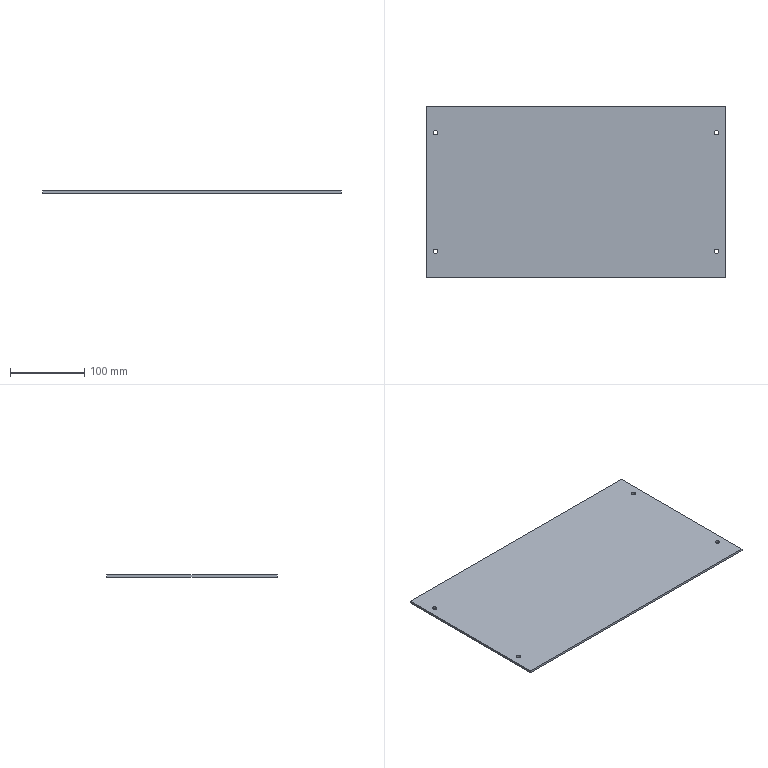Part | STEP file | Guard 7 | 1 solid | 14 faces | box 402 x 230 x 3 mm | volume 277041 mm3 | cylinder 8 | plane 6 | commonest cylinder face diameters 6 x8
STEP:
#1=CARTESIAN_POINT('',(192.,-80.,0.));
#2=VERTEX_POINT('',#1);
#3=CARTESIAN_POINT('',(186.,-80.,0.));
#4=VERTEX_POINT('',#3);
#5=CARTESIAN_POINT('',(189.,-80.,0.));
#6=DIRECTION('',(0.,0.,-1.));
#7=DIRECTION('',(1.,0.,0.));
#8=AXIS2_PLACEMENT_3D('',#5,#6,#7);
#9=CIRCLE('',#8,3.);
#10=EDGE_CURVE('',#2,#4,#9,.T.);
#11=ORIENTED_EDGE('',*,*,#10,.T.);
#12=CARTESIAN_POINT('',(186.,-80.,3.));
#13=VERTEX_POINT('',#12);
#14=CARTESIAN_POINT('',(186.,-80.,-7.));
#15=DIRECTION('',(0.,0.,1.));
#16=VECTOR('',#15,1000.);
#17=LINE('',#14,#16);
#18=EDGE_CURVE('',#4,#13,#17,.T.);
#19=ORIENTED_EDGE('',*,*,#18,.T.);
#20=CARTESIAN_POINT('',(192.,-80.,3.));
#21=VERTEX_POINT('',#20);
#22=CARTESIAN_POINT('',(189.,-80.,3.));
#23=DIRECTION('',(0.,0.,-1.));
#24=DIRECTION('',(-1.,0.,0.));
#25=AXIS2_PLACEMENT_3D('',#22,#23,#24);
#26=CIRCLE('',#25,3.);
#27=EDGE_CURVE('',#21,#13,#26,.T.);
#28=ORIENTED_EDGE('',*,*,#27,.F.);
#29=CARTESIAN_POINT('',(192.,-80.,-7.));
#30=DIRECTION('',(0.,0.,1.));
#31=VECTOR('',#30,1000.);
#32=LINE('',#29,#31);
#33=EDGE_CURVE('',#2,#21,#32,.T.);
#34=ORIENTED_EDGE('',*,*,#33,.F.);
#35=EDGE_LOOP('',(#11,#19,#28,#34));
#36=FACE_OUTER_BOUND('',#35,.T.);
#37=CARTESIAN_POINT('',(189.,-80.,-7.));
#38=DIRECTION('',(0.,0.,1.));
#39=DIRECTION('',(1.,0.,0.));
#40=AXIS2_PLACEMENT_3D('',#37,#38,#39);
#41=CYLINDRICAL_SURFACE('',#40,3.);
#42=ADVANCED_FACE('',(#36),#41,.F.);
#43=CARTESIAN_POINT('',(192.,80.,0.));
#44=VERTEX_POINT('',#43);
#45=CARTESIAN_POINT('',(186.,80.,0.));
#46=VERTEX_POINT('',#45);
#47=CARTESIAN_POINT('',(189.,80.,0.));
#48=DIRECTION('',(0.,0.,-1.));
#49=DIRECTION('',(1.,0.,0.));
#50=AXIS2_PLACEMENT_3D('',#47,#48,#49);
#51=CIRCLE('',#50,3.);
#52=EDGE_CURVE('',#44,#46,#51,.T.);
#53=ORIENTED_EDGE('',*,*,#52,.T.);
#54=CARTESIAN_POINT('',(186.,80.,3.));
#55=VERTEX_POINT('',#54);
#56=CARTESIAN_POINT('',(186.,80.,-7.));
#57=DIRECTION('',(0.,0.,1.));
#58=VECTOR('',#57,1000.);
#59=LINE('',#56,#58);
#60=EDGE_CURVE('',#46,#55,#59,.T.);
#61=ORIENTED_EDGE('',*,*,#60,.T.);
#62=CARTESIAN_POINT('',(192.,80.,3.));
#63=VERTEX_POINT('',#62);
#64=CARTESIAN_POINT('',(189.,80.,3.));
#65=DIRECTION('',(0.,0.,-1.));
#66=DIRECTION('',(-1.,0.,0.));
#67=AXIS2_PLACEMENT_3D('',#64,#65,#66);
#68=CIRCLE('',#67,3.);
#69=EDGE_CURVE('',#63,#55,#68,.T.);
#70=ORIENTED_EDGE('',*,*,#69,.F.);
#71=CARTESIAN_POINT('',(192.,80.,-7.));
#72=DIRECTION('',(0.,0.,1.));
#73=VECTOR('',#72,1000.);
#74=LINE('',#71,#73);
#75=EDGE_CURVE('',#44,#63,#74,.T.);
#76=ORIENTED_EDGE('',*,*,#75,.F.);
#77=EDGE_LOOP('',(#53,#61,#70,#76));
#78=FACE_OUTER_BOUND('',#77,.T.);
#79=CARTESIAN_POINT('',(189.,80.,-7.));
#80=DIRECTION('',(0.,0.,1.));
#81=DIRECTION('',(1.,0.,0.));
#82=AXIS2_PLACEMENT_3D('',#79,#80,#81);
#83=CYLINDRICAL_SURFACE('',#82,3.);
#84=ADVANCED_FACE('',(#78),#83,.F.);
#85=CARTESIAN_POINT('',(-192.,-80.,0.));
#86=VERTEX_POINT('',#85);
#87=CARTESIAN_POINT('',(-186.,-80.,0.));
#88=VERTEX_POINT('',#87);
#89=CARTESIAN_POINT('',(-189.,-80.,0.));
#90=DIRECTION('',(0.,0.,1.));
#91=DIRECTION('',(1.,0.,0.));
#92=AXIS2_PLACEMENT_3D('',#89,#90,#91);
#93=CIRCLE('',#92,3.);
#94=EDGE_CURVE('',#86,#88,#93,.T.);
#95=ORIENTED_EDGE('',*,*,#94,.F.);
#96=CARTESIAN_POINT('',(-192.,-80.,3.));
#97=VERTEX_POINT('',#96);
#98=CARTESIAN_POINT('',(-192.,-80.,-7.));
#99=DIRECTION('',(0.,0.,1.));
#100=VECTOR('',#99,1000.);
#101=LINE('',#98,#100);
#102=EDGE_CURVE('',#86,#97,#101,.T.);
#103=ORIENTED_EDGE('',*,*,#102,.T.);
#104=CARTESIAN_POINT('',(-186.,-80.,3.));
#105=VERTEX_POINT('',#104);
#106=CARTESIAN_POINT('',(-189.,-80.,3.));
#107=DIRECTION('',(0.,0.,1.));
#108=DIRECTION('',(1.,0.,0.));
#109=AXIS2_PLACEMENT_3D('',#106,#107,#108);
#110=CIRCLE('',#109,3.);
#111=EDGE_CURVE('',#97,#105,#110,.T.);
#112=ORIENTED_EDGE('',*,*,#111,.T.);
#113=CARTESIAN_POINT('',(-186.,-80.,-7.));
#114=DIRECTION('',(0.,0.,1.));
#115=VECTOR('',#114,1000.);
#116=LINE('',#113,#115);
#117=EDGE_CURVE('',#88,#105,#116,.T.);
#118=ORIENTED_EDGE('',*,*,#117,.F.);
#119=EDGE_LOOP('',(#95,#103,#112,#118));
#120=FACE_OUTER_BOUND('',#119,.T.);
#121=CARTESIAN_POINT('',(-189.,-80.,-7.));
#122=DIRECTION('',(0.,0.,1.));
#123=DIRECTION('',(1.,0.,0.));
#124=AXIS2_PLACEMENT_3D('',#121,#122,#123);
#125=CYLINDRICAL_SURFACE('',#124,3.);
#126=ADVANCED_FACE('',(#120),#125,.F.);
#127=CARTESIAN_POINT('',(-192.,80.,0.));
#128=VERTEX_POINT('',#127);
#129=CARTESIAN_POINT('',(-186.,80.,0.));
#130=VERTEX_POINT('',#129);
#131=CARTESIAN_POINT('',(-189.,80.,0.));
#132=DIRECTION('',(0.,0.,1.));
#133=DIRECTION('',(1.,0.,0.));
#134=AXIS2_PLACEMENT_3D('',#131,#132,#133);
#135=CIRCLE('',#134,3.);
#136=EDGE_CURVE('',#128,#130,#135,.T.);
#137=ORIENTED_EDGE('',*,*,#136,.F.);
#138=CARTESIAN_POINT('',(-192.,80.,3.));
#139=VERTEX_POINT('',#138);
#140=CARTESIAN_POINT('',(-192.,80.,-7.));
#141=DIRECTION('',(0.,0.,1.));
#142=VECTOR('',#141,1000.);
#143=LINE('',#140,#142);
#144=EDGE_CURVE('',#128,#139,#143,.T.);
#145=ORIENTED_EDGE('',*,*,#144,.T.);
#146=CARTESIAN_POINT('',(-186.,80.,3.));
#147=VERTEX_POINT('',#146);
#148=CARTESIAN_POINT('',(-189.,80.,3.));
#149=DIRECTION('',(0.,0.,1.));
#150=DIRECTION('',(1.,0.,0.));
#151=AXIS2_PLACEMENT_3D('',#148,#149,#150);
#152=CIRCLE('',#151,3.);
#153=EDGE_CURVE('',#139,#147,#152,.T.);
#154=ORIENTED_EDGE('',*,*,#153,.T.);
#155=CARTESIAN_POINT('',(-186.,80.,-7.));
#156=DIRECTION('',(0.,0.,1.));
#157=VECTOR('',#156,1000.);
#158=LINE('',#155,#157);
#159=EDGE_CURVE('',#130,#147,#158,.T.);
#160=ORIENTED_EDGE('',*,*,#159,.F.);
#161=EDGE_LOOP('',(#137,#145,#154,#160));
#162=FACE_OUTER_BOUND('',#161,.T.);
#163=CARTESIAN_POINT('',(-189.,80.,-7.));
#164=DIRECTION('',(0.,0.,1.));
#165=DIRECTION('',(1.,0.,0.));
#166=AXIS2_PLACEMENT_3D('',#163,#164,#165);
#167=CYLINDRICAL_SURFACE('',#166,3.);
#168=ADVANCED_FACE('',(#162),#167,.F.);
#169=CARTESIAN_POINT('',(201.,-115.,0.));
#170=VERTEX_POINT('',#169);
#171=CARTESIAN_POINT('',(201.,115.,0.));
#172=VERTEX_POINT('',#171);
#173=CARTESIAN_POINT('',(201.,115.,0.));
#174=DIRECTION('',(0.,1.,0.));
#175=VECTOR('',#174,1000.);
#176=LINE('',#173,#175);
#177=EDGE_CURVE('',#170,#172,#176,.T.);
#178=ORIENTED_EDGE('',*,*,#177,.T.);
#179=CARTESIAN_POINT('',(201.,115.,3.));
#180=VERTEX_POINT('',#179);
#181=CARTESIAN_POINT('',(201.,115.,3.));
#182=DIRECTION('',(0.,0.,-1.));
#183=VECTOR('',#182,1000.);
#184=LINE('',#181,#183);
#185=EDGE_CURVE('',#180,#172,#184,.T.);
#186=ORIENTED_EDGE('',*,*,#185,.F.);
#187=CARTESIAN_POINT('',(201.,-115.,3.));
#188=VERTEX_POINT('',#187);
#189=CARTESIAN_POINT('',(201.,115.,3.));
#190=DIRECTION('',(0.,1.,0.));
#191=VECTOR('',#190,1000.);
#192=LINE('',#189,#191);
#193=EDGE_CURVE('',#188,#180,#192,.T.);
#194=ORIENTED_EDGE('',*,*,#193,.F.);
#195=CARTESIAN_POINT('',(201.,-115.,3.));
#196=DIRECTION('',(0.,0.,-1.));
#197=VECTOR('',#196,1000.);
#198=LINE('',#195,#197);
#199=EDGE_CURVE('',#188,#170,#198,.T.);
#200=ORIENTED_EDGE('',*,*,#199,.T.);
#201=EDGE_LOOP('',(#178,#186,#194,#200));
#202=FACE_OUTER_BOUND('',#201,.T.);
#203=CARTESIAN_POINT('',(201.,115.,3.));
#204=DIRECTION('',(-1.,0.,0.));
#205=DIRECTION('',(0.,0.,1.));
#206=AXIS2_PLACEMENT_3D('',#203,#204,#205);
#207=PLANE('',#206);
#208=ADVANCED_FACE('',(#202),#207,.F.);
#209=CARTESIAN_POINT('',(-201.,115.,0.));
#210=VERTEX_POINT('',#209);
#211=CARTESIAN_POINT('',(-201.,115.,0.));
#212=DIRECTION('',(-1.,0.,0.));
#213=VECTOR('',#212,1000.);
#214=LINE('',#211,#213);
#215=EDGE_CURVE('',#172,#210,#214,.T.);
#216=ORIENTED_EDGE('',*,*,#215,.T.);
#217=CARTESIAN_POINT('',(-201.,115.,3.));
#218=VERTEX_POINT('',#217);
#219=CARTESIAN_POINT('',(-201.,115.,3.));
#220=DIRECTION('',(0.,0.,-1.));
#221=VECTOR('',#220,1000.);
#222=LINE('',#219,#221);
#223=EDGE_CURVE('',#218,#210,#222,.T.);
#224=ORIENTED_EDGE('',*,*,#223,.F.);
#225=CARTESIAN_POINT('',(-201.,115.,3.));
#226=DIRECTION('',(-1.,0.,0.));
#227=VECTOR('',#226,1000.);
#228=LINE('',#225,#227);
#229=EDGE_CURVE('',#180,#218,#228,.T.);
#230=ORIENTED_EDGE('',*,*,#229,.F.);
#231=ORIENTED_EDGE('',*,*,#185,.T.);
#232=EDGE_LOOP('',(#216,#224,#230,#231));
#233=FACE_OUTER_BOUND('',#232,.T.);
#234=CARTESIAN_POINT('',(-201.,115.,3.));
#235=DIRECTION('',(0.,-1.,0.));
#236=DIRECTION('',(0.,0.,-1.));
#237=AXIS2_PLACEMENT_3D('',#234,#235,#236);
#238=PLANE('',#237);
#239=ADVANCED_FACE('',(#233),#238,.F.);
#240=CARTESIAN_POINT('',(-201.,-115.,0.));
#241=VERTEX_POINT('',#240);
#242=CARTESIAN_POINT('',(-201.,115.,0.));
#243=DIRECTION('',(0.,-1.,0.));
#244=VECTOR('',#243,1000.);
#245=LINE('',#242,#244);
#246=EDGE_CURVE('',#210,#241,#245,.T.);
#247=ORIENTED_EDGE('',*,*,#246,.T.);
#248=CARTESIAN_POINT('',(-201.,-115.,3.));
#249=VERTEX_POINT('',#248);
#250=CARTESIAN_POINT('',(-201.,-115.,3.));
#251=DIRECTION('',(0.,0.,-1.));
#252=VECTOR('',#251,1000.);
#253=LINE('',#250,#252);
#254=EDGE_CURVE('',#249,#241,#253,.T.);
#255=ORIENTED_EDGE('',*,*,#254,.F.);
#256=CARTESIAN_POINT('',(-201.,115.,3.));
#257=DIRECTION('',(0.,-1.,0.));
#258=VECTOR('',#257,1000.);
#259=LINE('',#256,#258);
#260=EDGE_CURVE('',#218,#249,#259,.T.);
#261=ORIENTED_EDGE('',*,*,#260,.F.);
#262=ORIENTED_EDGE('',*,*,#223,.T.);
#263=EDGE_LOOP('',(#247,#255,#261,#262));
#264=FACE_OUTER_BOUND('',#263,.T.);
#265=CARTESIAN_POINT('',(-201.,115.,3.));
#266=DIRECTION('',(1.,0.,0.));
#267=DIRECTION('',(0.,0.,-1.));
#268=AXIS2_PLACEMENT_3D('',#265,#266,#267);
#269=PLANE('',#268);
#270=ADVANCED_FACE('',(#264),#269,.F.);
#271=CARTESIAN_POINT('',(-201.,-115.,0.));
#272=DIRECTION('',(1.,0.,0.));
#273=VECTOR('',#272,1000.);
#274=LINE('',#271,#273);
#275=EDGE_CURVE('',#241,#170,#274,.T.);
#276=ORIENTED_EDGE('',*,*,#275,.T.);
#277=ORIENTED_EDGE('',*,*,#199,.F.);
#278=CARTESIAN_POINT('',(-201.,-115.,3.));
#279=DIRECTION('',(1.,0.,0.));
#280=VECTOR('',#279,1000.);
#281=LINE('',#278,#280);
#282=EDGE_CURVE('',#249,#188,#281,.T.);
#283=ORIENTED_EDGE('',*,*,#282,.F.);
#284=ORIENTED_EDGE('',*,*,#254,.T.);
#285=EDGE_LOOP('',(#276,#277,#283,#284));
#286=FACE_OUTER_BOUND('',#285,.T.);
#287=CARTESIAN_POINT('',(-201.,-115.,3.));
#288=DIRECTION('',(0.,1.,0.));
#289=DIRECTION('',(0.,0.,1.));
#290=AXIS2_PLACEMENT_3D('',#287,#288,#289);
#291=PLANE('',#290);
#292=ADVANCED_FACE('',(#286),#291,.F.);
#293=ORIENTED_EDGE('',*,*,#27,.T.);
#294=CARTESIAN_POINT('',(189.,-80.,3.));
#295=DIRECTION('',(0.,0.,-1.));
#296=DIRECTION('',(-1.,0.,0.));
#297=AXIS2_PLACEMENT_3D('',#294,#295,#296);
#298=CIRCLE('',#297,3.);
#299=EDGE_CURVE('',#13,#21,#298,.T.);
#300=ORIENTED_EDGE('',*,*,#299,.T.);
#301=EDGE_LOOP('',(#293,#300));
#302=FACE_BOUND('',#301,.T.);
#303=ORIENTED_EDGE('',*,*,#69,.T.);
#304=CARTESIAN_POINT('',(189.,80.,3.));
#305=DIRECTION('',(0.,0.,-1.));
#306=DIRECTION('',(-1.,0.,0.));
#307=AXIS2_PLACEMENT_3D('',#304,#305,#306);
#308=CIRCLE('',#307,3.);
#309=EDGE_CURVE('',#55,#63,#308,.T.);
#310=ORIENTED_EDGE('',*,*,#309,.T.);
#311=EDGE_LOOP('',(#303,#310));
#312=FACE_BOUND('',#311,.T.);
#313=CARTESIAN_POINT('',(-189.,-80.,3.));
#314=DIRECTION('',(0.,0.,1.));
#315=DIRECTION('',(1.,0.,0.));
#316=AXIS2_PLACEMENT_3D('',#313,#314,#315);
#317=CIRCLE('',#316,3.);
#318=EDGE_CURVE('',#105,#97,#317,.T.);
#319=ORIENTED_EDGE('',*,*,#318,.F.);
#320=ORIENTED_EDGE('',*,*,#111,.F.);
#321=EDGE_LOOP('',(#319,#320));
#322=FACE_BOUND('',#321,.T.);
#323=CARTESIAN_POINT('',(-189.,80.,3.));
#324=DIRECTION('',(0.,0.,1.));
#325=DIRECTION('',(1.,0.,0.));
#326=AXIS2_PLACEMENT_3D('',#323,#324,#325);
#327=CIRCLE('',#326,3.);
#328=EDGE_CURVE('',#147,#139,#327,.T.);
#329=ORIENTED_EDGE('',*,*,#328,.F.);
#330=ORIENTED_EDGE('',*,*,#153,.F.);
#331=EDGE_LOOP('',(#329,#330));
#332=FACE_BOUND('',#331,.T.);
#333=ORIENTED_EDGE('',*,*,#193,.T.);
#334=ORIENTED_EDGE('',*,*,#229,.T.);
#335=ORIENTED_EDGE('',*,*,#260,.T.);
#336=ORIENTED_EDGE('',*,*,#282,.T.);
#337=EDGE_LOOP('',(#333,#334,#335,#336));
#338=FACE_OUTER_BOUND('',#337,.T.);
#339=CARTESIAN_POINT('',(0.,0.,3.));
#340=DIRECTION('',(0.,0.,1.));
#341=DIRECTION('',(1.,0.,0.));
#342=AXIS2_PLACEMENT_3D('',#339,#340,#341);
#343=PLANE('',#342);
#344=ADVANCED_FACE('',(#302,#312,#322,#332,#338),#343,.T.);
#345=ORIENTED_EDGE('',*,*,#10,.F.);
#346=CARTESIAN_POINT('',(189.,-80.,0.));
#347=DIRECTION('',(0.,0.,-1.));
#348=DIRECTION('',(1.,0.,0.));
#349=AXIS2_PLACEMENT_3D('',#346,#347,#348);
#350=CIRCLE('',#349,3.);
#351=EDGE_CURVE('',#4,#2,#350,.T.);
#352=ORIENTED_EDGE('',*,*,#351,.F.);
#353=EDGE_LOOP('',(#345,#352));
#354=FACE_BOUND('',#353,.T.);
#355=ORIENTED_EDGE('',*,*,#52,.F.);
#356=CARTESIAN_POINT('',(189.,80.,0.));
#357=DIRECTION('',(0.,0.,-1.));
#358=DIRECTION('',(1.,0.,0.));
#359=AXIS2_PLACEMENT_3D('',#356,#357,#358);
#360=CIRCLE('',#359,3.);
#361=EDGE_CURVE('',#46,#44,#360,.T.);
#362=ORIENTED_EDGE('',*,*,#361,.F.);
#363=EDGE_LOOP('',(#355,#362));
#364=FACE_BOUND('',#363,.T.);
#365=CARTESIAN_POINT('',(-189.,-80.,0.));
#366=DIRECTION('',(0.,0.,1.));
#367=DIRECTION('',(1.,0.,0.));
#368=AXIS2_PLACEMENT_3D('',#365,#366,#367);
#369=CIRCLE('',#368,3.);
#370=EDGE_CURVE('',#88,#86,#369,.T.);
#371=ORIENTED_EDGE('',*,*,#370,.T.);
#372=ORIENTED_EDGE('',*,*,#94,.T.);
#373=EDGE_LOOP('',(#371,#372));
#374=FACE_BOUND('',#373,.T.);
#375=CARTESIAN_POINT('',(-189.,80.,0.));
#376=DIRECTION('',(0.,0.,1.));
#377=DIRECTION('',(1.,0.,0.));
#378=AXIS2_PLACEMENT_3D('',#375,#376,#377);
#379=CIRCLE('',#378,3.);
#380=EDGE_CURVE('',#130,#128,#379,.T.);
#381=ORIENTED_EDGE('',*,*,#380,.T.);
#382=ORIENTED_EDGE('',*,*,#136,.T.);
#383=EDGE_LOOP('',(#381,#382));
#384=FACE_BOUND('',#383,.T.);
#385=ORIENTED_EDGE('',*,*,#177,.F.);
#386=ORIENTED_EDGE('',*,*,#275,.F.);
#387=ORIENTED_EDGE('',*,*,#246,.F.);
#388=ORIENTED_EDGE('',*,*,#215,.F.);
#389=EDGE_LOOP('',(#385,#386,#387,#388));
#390=FACE_OUTER_BOUND('',#389,.T.);
#391=CARTESIAN_POINT('',(0.,0.,0.));
#392=DIRECTION('',(0.,0.,1.));
#393=DIRECTION('',(1.,0.,0.));
#394=AXIS2_PLACEMENT_3D('',#391,#392,#393);
#395=PLANE('',#394);
#396=ADVANCED_FACE('',(#354,#364,#374,#384,#390),#395,.F.);
#397=ORIENTED_EDGE('',*,*,#144,.F.);
#398=ORIENTED_EDGE('',*,*,#380,.F.);
#399=ORIENTED_EDGE('',*,*,#159,.T.);
#400=ORIENTED_EDGE('',*,*,#328,.T.);
#401=EDGE_LOOP('',(#397,#398,#399,#400));
#402=FACE_OUTER_BOUND('',#401,.T.);
#403=CARTESIAN_POINT('',(-189.,80.,-7.));
#404=DIRECTION('',(0.,0.,1.));
#405=DIRECTION('',(1.,0.,0.));
#406=AXIS2_PLACEMENT_3D('',#403,#404,#405);
#407=CYLINDRICAL_SURFACE('',#406,3.);
#408=ADVANCED_FACE('',(#402),#407,.F.);
#409=ORIENTED_EDGE('',*,*,#102,.F.);
#410=ORIENTED_EDGE('',*,*,#370,.F.);
#411=ORIENTED_EDGE('',*,*,#117,.T.);
#412=ORIENTED_EDGE('',*,*,#318,.T.);
#413=EDGE_LOOP('',(#409,#410,#411,#412));
#414=FACE_OUTER_BOUND('',#413,.T.);
#415=CARTESIAN_POINT('',(-189.,-80.,-7.));
#416=DIRECTION('',(0.,0.,1.));
#417=DIRECTION('',(1.,0.,0.));
#418=AXIS2_PLACEMENT_3D('',#415,#416,#417);
#419=CYLINDRICAL_SURFACE('',#418,3.);
#420=ADVANCED_FACE('',(#414),#419,.F.);
#421=ORIENTED_EDGE('',*,*,#60,.F.);
#422=ORIENTED_EDGE('',*,*,#361,.T.);
#423=ORIENTED_EDGE('',*,*,#75,.T.);
#424=ORIENTED_EDGE('',*,*,#309,.F.);
#425=EDGE_LOOP('',(#421,#422,#423,#424));
#426=FACE_OUTER_BOUND('',#425,.T.);
#427=CARTESIAN_POINT('',(189.,80.,-7.));
#428=DIRECTION('',(0.,0.,1.));
#429=DIRECTION('',(1.,0.,0.));
#430=AXIS2_PLACEMENT_3D('',#427,#428,#429);
#431=CYLINDRICAL_SURFACE('',#430,3.);
#432=ADVANCED_FACE('',(#426),#431,.F.);
#433=ORIENTED_EDGE('',*,*,#18,.F.);
#434=ORIENTED_EDGE('',*,*,#351,.T.);
#435=ORIENTED_EDGE('',*,*,#33,.T.);
#436=ORIENTED_EDGE('',*,*,#299,.F.);
#437=EDGE_LOOP('',(#433,#434,#435,#436));
#438=FACE_OUTER_BOUND('',#437,.T.);
#439=CARTESIAN_POINT('',(189.,-80.,-7.));
#440=DIRECTION('',(0.,0.,1.));
#441=DIRECTION('',(1.,0.,0.));
#442=AXIS2_PLACEMENT_3D('',#439,#440,#441);
#443=CYLINDRICAL_SURFACE('',#442,3.);
#444=ADVANCED_FACE('',(#438),#443,.F.);
#445=CLOSED_SHELL('',(#42,#84,#126,#168,#208,#239,#270,#292,#344,#396,#408,#420,#432,#444));
#446=MANIFOLD_SOLID_BREP('',#445);
#447=CARTESIAN_POINT('',(0.,0.,0.));
#448=DIRECTION('',(0.,0.,1.));
#449=DIRECTION('',(1.,0.,0.));
#450=AXIS2_PLACEMENT_3D('',#447,#448,#449);
#451=(LENGTH_UNIT()NAMED_UNIT(*)SI_UNIT(.MILLI.,.METRE.));
#452=UNCERTAINTY_MEASURE_WITH_UNIT(LENGTH_MEASURE(0.00001),#451,'','');
#453=(NAMED_UNIT(*)PLANE_ANGLE_UNIT()SI_UNIT($,.RADIAN.));
#454=(NAMED_UNIT(*)SI_UNIT($,.STERADIAN.)SOLID_ANGLE_UNIT());
#455=(GEOMETRIC_REPRESENTATION_CONTEXT(3)GLOBAL_UNCERTAINTY_ASSIGNED_CONTEXT((#452))GLOBAL_UNIT_ASSIGNED_CONTEXT((#451,#453,#454))REPRESENTATION_CONTEXT('',''));
#456=ADVANCED_BREP_SHAPE_REPRESENTATION('',(#446,#450),#455);